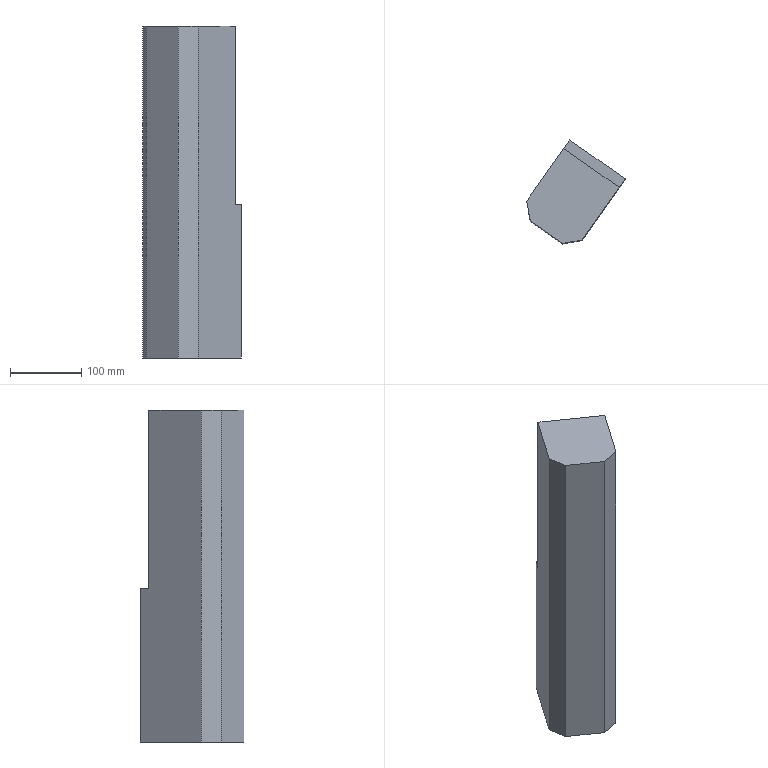Part | NX | features solid 2 | 1 solid | 22 faces | box 138.045 x 145.412 x 465 mm | volume 4926060 mm3 | plane 12 | cylinder 6 | cone 4 | commonest cylinder face diameters 16 x6
STEP:
#1=CARTESIAN_POINT('',(-184.572,-199.868,-589.062));
#2=VERTEX_POINT('',#1);
#3=CARTESIAN_POINT('',(-176.572,-199.868,-589.062));
#4=DIRECTION('',(0.,0.,-1.));
#5=DIRECTION('',(-1.,0.,0.));
#6=AXIS2_PLACEMENT_3D('',#3,#4,#5);
#7=CIRCLE('',#6,8.);
#8=EDGE_CURVE('',#2,#2,#7,.T.);
#9=ORIENTED_EDGE('',*,*,#8,.F.);
#10=EDGE_LOOP('',(#9));
#11=FACE_BOUND('',#10,.T.);
#12=CARTESIAN_POINT('',(-199.286,-147.842,-589.062));
#13=VERTEX_POINT('',#12);
#14=CARTESIAN_POINT('',(-207.286,-147.842,-589.062));
#15=DIRECTION('',(0.,0.,1.));
#16=DIRECTION('',(1.,0.,0.));
#17=AXIS2_PLACEMENT_3D('',#14,#15,#16);
#18=CIRCLE('',#17,8.);
#19=EDGE_CURVE('',#13,#13,#18,.T.);
#20=ORIENTED_EDGE('',*,*,#19,.T.);
#21=EDGE_LOOP('',(#20));
#22=FACE_BOUND('',#21,.T.);
#23=CARTESIAN_POINT('',(-236.569,-201.087,-589.062));
#24=VERTEX_POINT('',#23);
#25=CARTESIAN_POINT('',(-244.569,-201.087,-589.062));
#26=DIRECTION('',(0.,0.,1.));
#27=DIRECTION('',(1.,0.,0.));
#28=AXIS2_PLACEMENT_3D('',#25,#26,#27);
#29=CIRCLE('',#28,8.);
#30=EDGE_CURVE('',#24,#24,#29,.T.);
#31=ORIENTED_EDGE('',*,*,#30,.T.);
#32=EDGE_LOOP('',(#31));
#33=FACE_BOUND('',#32,.T.);
#34=CARTESIAN_POINT('',(-154.233,-179.389,-589.062));
#35=VERTEX_POINT('',#34);
#36=CARTESIAN_POINT('',(-162.233,-179.389,-589.062));
#37=DIRECTION('',(0.,0.,1.));
#38=DIRECTION('',(1.,0.,0.));
#39=AXIS2_PLACEMENT_3D('',#36,#37,#38);
#40=CIRCLE('',#39,8.);
#41=EDGE_CURVE('',#35,#35,#40,.T.);
#42=ORIENTED_EDGE('',*,*,#41,.T.);
#43=EDGE_LOOP('',(#42));
#44=FACE_BOUND('',#43,.T.);
#45=CARTESIAN_POINT('',(-191.515,-232.634,-589.062));
#46=VERTEX_POINT('',#45);
#47=CARTESIAN_POINT('',(-199.515,-232.634,-589.062));
#48=DIRECTION('',(0.,0.,1.));
#49=DIRECTION('',(1.,0.,0.));
#50=AXIS2_PLACEMENT_3D('',#47,#48,#49);
#51=CIRCLE('',#50,8.);
#52=EDGE_CURVE('',#46,#46,#51,.T.);
#53=ORIENTED_EDGE('',*,*,#52,.T.);
#54=EDGE_LOOP('',(#53));
#55=FACE_BOUND('',#54,.T.);
#56=CARTESIAN_POINT('',(-128.643,-166.286,-589.062));
#57=VERTEX_POINT('',#56);
#58=CARTESIAN_POINT('',(-188.868,-252.297,-589.062));
#59=VERTEX_POINT('',#58);
#60=CARTESIAN_POINT('',(-197.472,-264.584,-589.062));
#61=DIRECTION('',(-0.5736,-0.8192,0.));
#62=VECTOR('',#61,1000.);
#63=LINE('',#60,#62);
#64=EDGE_CURVE('',#57,#59,#63,.T.);
#65=ORIENTED_EDGE('',*,*,#64,.T.);
#66=CARTESIAN_POINT('',(-216.723,-257.209,-589.062));
#67=VERTEX_POINT('',#66);
#68=CARTESIAN_POINT('',(-188.868,-252.297,-589.062));
#69=DIRECTION('',(0.9848,0.1736,0.));
#70=VECTOR('',#69,1000.);
#71=LINE('',#68,#70);
#72=EDGE_CURVE('',#59,#67,#71,.F.);
#73=ORIENTED_EDGE('',*,*,#72,.T.);
#74=CARTESIAN_POINT('',(-261.776,-225.662,-589.062));
#75=VERTEX_POINT('',#74);
#76=CARTESIAN_POINT('',(-278.241,-214.133,-589.062));
#77=DIRECTION('',(0.8192,-0.5736,0.));
#78=VECTOR('',#77,1000.);
#79=LINE('',#76,#78);
#80=EDGE_CURVE('',#67,#75,#79,.F.);
#81=ORIENTED_EDGE('',*,*,#80,.T.);
#82=CARTESIAN_POINT('',(-266.688,-197.807,-589.062));
#83=VERTEX_POINT('',#82);
#84=CARTESIAN_POINT('',(-261.776,-225.662,-589.062));
#85=DIRECTION('',(0.1736,-0.9848,0.));
#86=VECTOR('',#85,1000.);
#87=LINE('',#84,#86);
#88=EDGE_CURVE('',#75,#83,#87,.F.);
#89=ORIENTED_EDGE('',*,*,#88,.T.);
#90=CARTESIAN_POINT('',(-206.462,-111.796,-589.062));
#91=VERTEX_POINT('',#90);
#92=CARTESIAN_POINT('',(-275.291,-210.095,-589.062));
#93=DIRECTION('',(0.5736,0.8192,0.));
#94=VECTOR('',#93,1000.);
#95=LINE('',#92,#94);
#96=EDGE_CURVE('',#91,#83,#95,.F.);
#97=ORIENTED_EDGE('',*,*,#96,.F.);
#98=CARTESIAN_POINT('',(-206.544,-111.739,-589.062));
#99=DIRECTION('',(0.8192,-0.5736,0.));
#100=VECTOR('',#99,1000.);
#101=LINE('',#98,#100);
#102=EDGE_CURVE('',#57,#91,#101,.F.);
#103=ORIENTED_EDGE('',*,*,#102,.F.);
#104=EDGE_LOOP('',(#65,#73,#81,#89,#97,#103));
#105=FACE_BOUND('',#104,.T.);
#106=CARTESIAN_POINT('',(-238.229,-180.609,-589.062));
#107=VERTEX_POINT('',#106);
#108=CARTESIAN_POINT('',(-230.229,-180.609,-589.062));
#109=DIRECTION('',(0.,0.,-1.));
#110=DIRECTION('',(-1.,0.,0.));
#111=AXIS2_PLACEMENT_3D('',#108,#109,#110);
#112=CIRCLE('',#111,8.);
#113=EDGE_CURVE('',#107,#107,#112,.T.);
#114=ORIENTED_EDGE('',*,*,#113,.F.);
#115=EDGE_LOOP('',(#114));
#116=FACE_BOUND('',#115,.T.);
#117=CARTESIAN_POINT('',(-275.373,-210.037,-589.062));
#118=DIRECTION('',(0.,0.,-1.));
#119=DIRECTION('',(0.5736,0.8192,0.));
#120=AXIS2_PLACEMENT_3D('',#117,#118,#119);
#121=PLANE('',#120);
#122=ADVANCED_FACE('',(#11,#22,#33,#44,#55,#105,#116),#121,.T.);
#123=CARTESIAN_POINT('',(-261.776,-225.662,-124.062));
#124=VERTEX_POINT('',#123);
#125=CARTESIAN_POINT('',(-216.723,-257.209,-124.062));
#126=VERTEX_POINT('',#125);
#127=CARTESIAN_POINT('',(-278.159,-214.19,-124.062));
#128=DIRECTION('',(0.8192,-0.5736,0.));
#129=VECTOR('',#128,1000.);
#130=LINE('',#127,#129);
#131=EDGE_CURVE('',#124,#126,#130,.T.);
#132=ORIENTED_EDGE('',*,*,#131,.T.);
#133=CARTESIAN_POINT('',(-188.868,-252.297,-124.062));
#134=VERTEX_POINT('',#133);
#135=CARTESIAN_POINT('',(-188.868,-252.297,-124.062));
#136=DIRECTION('',(0.9848,0.1736,0.));
#137=VECTOR('',#136,1000.);
#138=LINE('',#135,#137);
#139=EDGE_CURVE('',#126,#134,#138,.T.);
#140=ORIENTED_EDGE('',*,*,#139,.T.);
#141=CARTESIAN_POINT('',(-137.246,-178.573,-124.062));
#142=VERTEX_POINT('',#141);
#143=CARTESIAN_POINT('',(-48.342,-51.605,-124.062));
#144=DIRECTION('',(0.5736,0.8192,0.));
#145=VECTOR('',#144,1000.);
#146=LINE('',#143,#145);
#147=EDGE_CURVE('',#142,#134,#146,.F.);
#148=ORIENTED_EDGE('',*,*,#147,.F.);
#149=CARTESIAN_POINT('',(-215.066,-124.084,-124.062));
#150=VERTEX_POINT('',#149);
#151=CARTESIAN_POINT('',(-215.066,-124.084,-124.062));
#152=DIRECTION('',(0.8192,-0.5736,0.));
#153=VECTOR('',#152,1000.);
#154=LINE('',#151,#153);
#155=EDGE_CURVE('',#150,#142,#154,.T.);
#156=ORIENTED_EDGE('',*,*,#155,.F.);
#157=CARTESIAN_POINT('',(-266.688,-197.807,-124.062));
#158=VERTEX_POINT('',#157);
#159=CARTESIAN_POINT('',(-215.066,-124.084,-124.062));
#160=DIRECTION('',(-0.5736,-0.8192,0.));
#161=VECTOR('',#160,1000.);
#162=LINE('',#159,#161);
#163=EDGE_CURVE('',#150,#158,#162,.T.);
#164=ORIENTED_EDGE('',*,*,#163,.T.);
#165=CARTESIAN_POINT('',(-261.776,-225.662,-124.062));
#166=DIRECTION('',(0.1736,-0.9848,0.));
#167=VECTOR('',#166,1000.);
#168=LINE('',#165,#167);
#169=EDGE_CURVE('',#158,#124,#168,.T.);
#170=ORIENTED_EDGE('',*,*,#169,.T.);
#171=EDGE_LOOP('',(#132,#140,#148,#156,#164,#170));
#172=FACE_BOUND('',#171,.T.);
#173=CARTESIAN_POINT('',(-215.066,-124.084,-124.062));
#174=DIRECTION('',(0.,0.,-1.));
#175=DIRECTION('',(-0.5736,-0.8192,0.));
#176=AXIS2_PLACEMENT_3D('',#173,#174,#175);
#177=PLANE('',#176);
#178=ADVANCED_FACE('',(#172),#177,.F.);
#179=CARTESIAN_POINT('',(-137.246,-178.573,-374.062));
#180=VERTEX_POINT('',#179);
#181=CARTESIAN_POINT('',(-137.246,-178.573,-401.082));
#182=DIRECTION('',(0.,0.,1.));
#183=VECTOR('',#182,1000.);
#184=LINE('',#181,#183);
#185=EDGE_CURVE('',#142,#180,#184,.F.);
#186=ORIENTED_EDGE('',*,*,#185,.T.);
#187=CARTESIAN_POINT('',(-215.066,-124.084,-374.062));
#188=VERTEX_POINT('',#187);
#189=CARTESIAN_POINT('',(-215.066,-124.084,-374.062));
#190=DIRECTION('',(-0.8192,0.5736,0.));
#191=VECTOR('',#190,1000.);
#192=LINE('',#189,#191);
#193=EDGE_CURVE('',#180,#188,#192,.T.);
#194=ORIENTED_EDGE('',*,*,#193,.T.);
#195=CARTESIAN_POINT('',(-215.066,-124.084,-401.082));
#196=DIRECTION('',(0.,0.,-1.));
#197=VECTOR('',#196,1000.);
#198=LINE('',#195,#197);
#199=EDGE_CURVE('',#150,#188,#198,.T.);
#200=ORIENTED_EDGE('',*,*,#199,.F.);
#201=ORIENTED_EDGE('',*,*,#155,.T.);
#202=EDGE_LOOP('',(#186,#194,#200,#201));
#203=FACE_BOUND('',#202,.T.);
#204=CARTESIAN_POINT('',(-215.066,-124.084,-401.082));
#205=DIRECTION('',(-0.5736,-0.8192,0.));
#206=DIRECTION('',(0.8192,-0.5736,0.));
#207=AXIS2_PLACEMENT_3D('',#204,#205,#206);
#208=PLANE('',#207);
#209=ADVANCED_FACE('',(#203),#208,.F.);
#210=CARTESIAN_POINT('',(-128.643,-166.286,-374.062));
#211=VERTEX_POINT('',#210);
#212=CARTESIAN_POINT('',(-206.462,-111.796,-374.062));
#213=VERTEX_POINT('',#212);
#214=CARTESIAN_POINT('',(-153.217,-149.079,-374.062));
#215=DIRECTION('',(-0.8192,0.5736,0.));
#216=VECTOR('',#215,1000.);
#217=LINE('',#214,#216);
#218=EDGE_CURVE('',#211,#213,#217,.T.);
#219=ORIENTED_EDGE('',*,*,#218,.F.);
#220=CARTESIAN_POINT('',(-128.643,-166.286,-400.));
#221=DIRECTION('',(0.,0.,1.));
#222=VECTOR('',#221,1000.);
#223=LINE('',#220,#222);
#224=EDGE_CURVE('',#211,#57,#223,.F.);
#225=ORIENTED_EDGE('',*,*,#224,.T.);
#226=ORIENTED_EDGE('',*,*,#102,.T.);
#227=CARTESIAN_POINT('',(-206.462,-111.796,-401.082));
#228=DIRECTION('',(0.,0.,-1.));
#229=VECTOR('',#228,1000.);
#230=LINE('',#227,#229);
#231=EDGE_CURVE('',#213,#91,#230,.T.);
#232=ORIENTED_EDGE('',*,*,#231,.F.);
#233=EDGE_LOOP('',(#219,#225,#226,#232));
#234=FACE_BOUND('',#233,.T.);
#235=CARTESIAN_POINT('',(-153.217,-149.079,-461.082));
#236=DIRECTION('',(0.5736,0.8192,0.));
#237=DIRECTION('',(-0.8192,0.5736,0.));
#238=AXIS2_PLACEMENT_3D('',#235,#236,#237);
#239=PLANE('',#238);
#240=ADVANCED_FACE('',(#234),#239,.T.);
#241=ORIENTED_EDGE('',*,*,#96,.T.);
#242=CARTESIAN_POINT('',(-266.688,-197.807,-151.082));
#243=DIRECTION('',(0.,0.,1.));
#244=VECTOR('',#243,1000.);
#245=LINE('',#242,#244);
#246=EDGE_CURVE('',#83,#158,#245,.T.);
#247=ORIENTED_EDGE('',*,*,#246,.T.);
#248=ORIENTED_EDGE('',*,*,#163,.F.);
#249=ORIENTED_EDGE('',*,*,#199,.T.);
#250=CARTESIAN_POINT('',(-215.066,-124.084,-374.062));
#251=DIRECTION('',(-0.5736,-0.8192,0.));
#252=VECTOR('',#251,1000.);
#253=LINE('',#250,#252);
#254=EDGE_CURVE('',#213,#188,#253,.T.);
#255=ORIENTED_EDGE('',*,*,#254,.F.);
#256=ORIENTED_EDGE('',*,*,#231,.T.);
#257=EDGE_LOOP('',(#241,#247,#248,#249,#255,#256));
#258=FACE_BOUND('',#257,.T.);
#259=CARTESIAN_POINT('',(-215.066,-124.084,-151.082));
#260=DIRECTION('',(-0.8192,0.5736,0.));
#261=DIRECTION('',(-0.5736,-0.8192,0.));
#262=AXIS2_PLACEMENT_3D('',#259,#260,#261);
#263=PLANE('',#262);
#264=ADVANCED_FACE('',(#258),#263,.T.);
#265=ORIENTED_EDGE('',*,*,#80,.F.);
#266=CARTESIAN_POINT('',(-216.723,-257.209,-192.696));
#267=DIRECTION('',(0.,0.,1.));
#268=VECTOR('',#267,1000.);
#269=LINE('',#266,#268);
#270=EDGE_CURVE('',#67,#126,#269,.T.);
#271=ORIENTED_EDGE('',*,*,#270,.T.);
#272=ORIENTED_EDGE('',*,*,#131,.F.);
#273=CARTESIAN_POINT('',(-261.776,-225.662,-589.062));
#274=DIRECTION('',(0.,0.,-1.));
#275=VECTOR('',#274,1000.);
#276=LINE('',#273,#275);
#277=EDGE_CURVE('',#124,#75,#276,.T.);
#278=ORIENTED_EDGE('',*,*,#277,.T.);
#279=EDGE_LOOP('',(#265,#271,#272,#278));
#280=FACE_BOUND('',#279,.T.);
#281=CARTESIAN_POINT('',(-789.915,144.145,-192.696));
#282=DIRECTION('',(0.5736,0.8192,0.));
#283=DIRECTION('',(-0.8192,0.5736,0.));
#284=AXIS2_PLACEMENT_3D('',#281,#282,#283);
#285=PLANE('',#284);
#286=ADVANCED_FACE('',(#280),#285,.F.);
#287=CARTESIAN_POINT('',(-137.246,-178.573,-374.062));
#288=DIRECTION('',(0.5736,0.8192,0.));
#289=VECTOR('',#288,1000.);
#290=LINE('',#287,#289);
#291=EDGE_CURVE('',#211,#180,#290,.F.);
#292=ORIENTED_EDGE('',*,*,#291,.F.);
#293=ORIENTED_EDGE('',*,*,#218,.T.);
#294=ORIENTED_EDGE('',*,*,#254,.T.);
#295=ORIENTED_EDGE('',*,*,#193,.F.);
#296=EDGE_LOOP('',(#292,#293,#294,#295));
#297=FACE_BOUND('',#296,.T.);
#298=CARTESIAN_POINT('',(-161.821,-161.366,-374.062));
#299=DIRECTION('',(0.,0.,1.));
#300=DIRECTION('',(0.5736,0.8192,0.));
#301=AXIS2_PLACEMENT_3D('',#298,#299,#300);
#302=PLANE('',#301);
#303=ADVANCED_FACE('',(#297),#302,.T.);
#304=ORIENTED_EDGE('',*,*,#185,.F.);
#305=ORIENTED_EDGE('',*,*,#147,.T.);
#306=CARTESIAN_POINT('',(-188.868,-252.297,-400.));
#307=DIRECTION('',(0.,0.,1.));
#308=VECTOR('',#307,1000.);
#309=LINE('',#306,#308);
#310=EDGE_CURVE('',#134,#59,#309,.F.);
#311=ORIENTED_EDGE('',*,*,#310,.T.);
#312=ORIENTED_EDGE('',*,*,#64,.F.);
#313=ORIENTED_EDGE('',*,*,#224,.F.);
#314=ORIENTED_EDGE('',*,*,#291,.T.);
#315=EDGE_LOOP('',(#304,#305,#311,#312,#313,#314));
#316=FACE_BOUND('',#315,.T.);
#317=CARTESIAN_POINT('',(-48.342,-51.605,-400.));
#318=DIRECTION('',(0.8192,-0.5736,0.));
#319=DIRECTION('',(0.,0.,1.));
#320=AXIS2_PLACEMENT_3D('',#317,#318,#319);
#321=PLANE('',#320);
#322=ADVANCED_FACE('',(#316),#321,.T.);
#323=ORIENTED_EDGE('',*,*,#169,.F.);
#324=ORIENTED_EDGE('',*,*,#246,.F.);
#325=ORIENTED_EDGE('',*,*,#88,.F.);
#326=ORIENTED_EDGE('',*,*,#277,.F.);
#327=EDGE_LOOP('',(#323,#324,#325,#326));
#328=FACE_BOUND('',#327,.T.);
#329=CARTESIAN_POINT('',(-261.776,-225.662,-192.696));
#330=DIRECTION('',(-0.9848,-0.1736,0.));
#331=DIRECTION('',(0.1736,-0.9848,0.));
#332=AXIS2_PLACEMENT_3D('',#329,#330,#331);
#333=PLANE('',#332);
#334=ADVANCED_FACE('',(#328),#333,.T.);
#335=ORIENTED_EDGE('',*,*,#139,.F.);
#336=ORIENTED_EDGE('',*,*,#270,.F.);
#337=ORIENTED_EDGE('',*,*,#72,.F.);
#338=ORIENTED_EDGE('',*,*,#310,.F.);
#339=EDGE_LOOP('',(#335,#336,#337,#338));
#340=FACE_BOUND('',#339,.T.);
#341=CARTESIAN_POINT('',(-188.868,-252.297,-400.));
#342=DIRECTION('',(0.1736,-0.9848,0.));
#343=DIRECTION('',(0.9848,0.1736,0.));
#344=AXIS2_PLACEMENT_3D('',#341,#342,#343);
#345=PLANE('',#344);
#346=ADVANCED_FACE('',(#340),#345,.T.);
#347=CARTESIAN_POINT('',(-191.515,-232.634,-539.062));
#348=VERTEX_POINT('',#347);
#349=CARTESIAN_POINT('',(-199.515,-232.634,-539.062));
#350=DIRECTION('',(0.,0.,1.));
#351=DIRECTION('',(1.,0.,0.));
#352=AXIS2_PLACEMENT_3D('',#349,#350,#351);
#353=CIRCLE('',#352,8.);
#354=EDGE_CURVE('',#348,#348,#353,.T.);
#355=ORIENTED_EDGE('',*,*,#354,.F.);
#356=EDGE_LOOP('',(#355));
#357=FACE_BOUND('',#356,.T.);
#358=CARTESIAN_POINT('',(-199.515,-232.634,-534.256));
#359=VERTEX_POINT('',#358);
#360=VERTEX_LOOP('',#359);
#361=FACE_BOUND('',#360,.T.);
#362=CARTESIAN_POINT('',(-199.515,-232.634,-539.062));
#363=DIRECTION('',(0.,0.,-1.));
#364=DIRECTION('',(-1.,0.,0.));
#365=AXIS2_PLACEMENT_3D('',#362,#363,#364);
#366=CONICAL_SURFACE('',#365,8.,1.03);
#367=ADVANCED_FACE('',(#357,#361),#366,.F.);
#368=ORIENTED_EDGE('',*,*,#354,.T.);
#369=EDGE_LOOP('',(#368));
#370=FACE_BOUND('',#369,.T.);
#371=ORIENTED_EDGE('',*,*,#52,.F.);
#372=EDGE_LOOP('',(#371));
#373=FACE_BOUND('',#372,.T.);
#374=CARTESIAN_POINT('',(-199.515,-232.634,-589.062));
#375=DIRECTION('',(0.,0.,1.));
#376=DIRECTION('',(1.,0.,0.));
#377=AXIS2_PLACEMENT_3D('',#374,#375,#376);
#378=CYLINDRICAL_SURFACE('',#377,8.);
#379=ADVANCED_FACE('',(#370,#373),#378,.F.);
#380=CARTESIAN_POINT('',(-154.233,-179.389,-539.062));
#381=VERTEX_POINT('',#380);
#382=CARTESIAN_POINT('',(-162.233,-179.389,-539.062));
#383=DIRECTION('',(0.,0.,1.));
#384=DIRECTION('',(1.,0.,0.));
#385=AXIS2_PLACEMENT_3D('',#382,#383,#384);
#386=CIRCLE('',#385,8.);
#387=EDGE_CURVE('',#381,#381,#386,.T.);
#388=ORIENTED_EDGE('',*,*,#387,.F.);
#389=EDGE_LOOP('',(#388));
#390=FACE_BOUND('',#389,.T.);
#391=CARTESIAN_POINT('',(-162.233,-179.389,-534.256));
#392=VERTEX_POINT('',#391);
#393=VERTEX_LOOP('',#392);
#394=FACE_BOUND('',#393,.T.);
#395=CARTESIAN_POINT('',(-162.233,-179.389,-539.062));
#396=DIRECTION('',(0.,0.,-1.));
#397=DIRECTION('',(-1.,0.,0.));
#398=AXIS2_PLACEMENT_3D('',#395,#396,#397);
#399=CONICAL_SURFACE('',#398,8.,1.03);
#400=ADVANCED_FACE('',(#390,#394),#399,.F.);
#401=ORIENTED_EDGE('',*,*,#387,.T.);
#402=EDGE_LOOP('',(#401));
#403=FACE_BOUND('',#402,.T.);
#404=ORIENTED_EDGE('',*,*,#41,.F.);
#405=EDGE_LOOP('',(#404));
#406=FACE_BOUND('',#405,.T.);
#407=CARTESIAN_POINT('',(-162.233,-179.389,-589.062));
#408=DIRECTION('',(0.,0.,1.));
#409=DIRECTION('',(1.,0.,0.));
#410=AXIS2_PLACEMENT_3D('',#407,#408,#409);
#411=CYLINDRICAL_SURFACE('',#410,8.);
#412=ADVANCED_FACE('',(#403,#406),#411,.F.);
#413=CARTESIAN_POINT('',(-236.569,-201.087,-539.062));
#414=VERTEX_POINT('',#413);
#415=CARTESIAN_POINT('',(-244.569,-201.087,-539.062));
#416=DIRECTION('',(0.,0.,1.));
#417=DIRECTION('',(1.,0.,0.));
#418=AXIS2_PLACEMENT_3D('',#415,#416,#417);
#419=CIRCLE('',#418,8.);
#420=EDGE_CURVE('',#414,#414,#419,.T.);
#421=ORIENTED_EDGE('',*,*,#420,.F.);
#422=EDGE_LOOP('',(#421));
#423=FACE_BOUND('',#422,.T.);
#424=CARTESIAN_POINT('',(-244.569,-201.087,-534.256));
#425=VERTEX_POINT('',#424);
#426=VERTEX_LOOP('',#425);
#427=FACE_BOUND('',#426,.T.);
#428=CARTESIAN_POINT('',(-244.569,-201.087,-539.062));
#429=DIRECTION('',(0.,0.,-1.));
#430=DIRECTION('',(-1.,0.,0.));
#431=AXIS2_PLACEMENT_3D('',#428,#429,#430);
#432=CONICAL_SURFACE('',#431,8.,1.03);
#433=ADVANCED_FACE('',(#423,#427),#432,.F.);
#434=ORIENTED_EDGE('',*,*,#420,.T.);
#435=EDGE_LOOP('',(#434));
#436=FACE_BOUND('',#435,.T.);
#437=ORIENTED_EDGE('',*,*,#30,.F.);
#438=EDGE_LOOP('',(#437));
#439=FACE_BOUND('',#438,.T.);
#440=CARTESIAN_POINT('',(-244.569,-201.087,-589.062));
#441=DIRECTION('',(0.,0.,1.));
#442=DIRECTION('',(1.,0.,0.));
#443=AXIS2_PLACEMENT_3D('',#440,#441,#442);
#444=CYLINDRICAL_SURFACE('',#443,8.);
#445=ADVANCED_FACE('',(#436,#439),#444,.F.);
#446=CARTESIAN_POINT('',(-199.286,-147.842,-539.062));
#447=VERTEX_POINT('',#446);
#448=CARTESIAN_POINT('',(-207.286,-147.842,-539.062));
#449=DIRECTION('',(0.,0.,1.));
#450=DIRECTION('',(1.,0.,0.));
#451=AXIS2_PLACEMENT_3D('',#448,#449,#450);
#452=CIRCLE('',#451,8.);
#453=EDGE_CURVE('',#447,#447,#452,.T.);
#454=ORIENTED_EDGE('',*,*,#453,.F.);
#455=EDGE_LOOP('',(#454));
#456=FACE_BOUND('',#455,.T.);
#457=CARTESIAN_POINT('',(-207.286,-147.842,-534.256));
#458=VERTEX_POINT('',#457);
#459=VERTEX_LOOP('',#458);
#460=FACE_BOUND('',#459,.T.);
#461=CARTESIAN_POINT('',(-207.286,-147.842,-539.062));
#462=DIRECTION('',(0.,0.,-1.));
#463=DIRECTION('',(-1.,0.,0.));
#464=AXIS2_PLACEMENT_3D('',#461,#462,#463);
#465=CONICAL_SURFACE('',#464,8.,1.03);
#466=ADVANCED_FACE('',(#456,#460),#465,.F.);
#467=ORIENTED_EDGE('',*,*,#453,.T.);
#468=EDGE_LOOP('',(#467));
#469=FACE_BOUND('',#468,.T.);
#470=ORIENTED_EDGE('',*,*,#19,.F.);
#471=EDGE_LOOP('',(#470));
#472=FACE_BOUND('',#471,.T.);
#473=CARTESIAN_POINT('',(-207.286,-147.842,-589.062));
#474=DIRECTION('',(0.,0.,1.));
#475=DIRECTION('',(1.,0.,0.));
#476=AXIS2_PLACEMENT_3D('',#473,#474,#475);
#477=CYLINDRICAL_SURFACE('',#476,8.);
#478=ADVANCED_FACE('',(#469,#472),#477,.F.);
#479=CARTESIAN_POINT('',(-184.572,-199.868,-559.062));
#480=VERTEX_POINT('',#479);
#481=CARTESIAN_POINT('',(-176.572,-199.868,-559.062));
#482=DIRECTION('',(0.,0.,-1.));
#483=DIRECTION('',(-1.,0.,0.));
#484=AXIS2_PLACEMENT_3D('',#481,#482,#483);
#485=CIRCLE('',#484,8.);
#486=EDGE_CURVE('',#480,#480,#485,.T.);
#487=ORIENTED_EDGE('',*,*,#486,.F.);
#488=EDGE_LOOP('',(#487));
#489=FACE_BOUND('',#488,.T.);
#490=ORIENTED_EDGE('',*,*,#8,.T.);
#491=EDGE_LOOP('',(#490));
#492=FACE_BOUND('',#491,.T.);
#493=CARTESIAN_POINT('',(-176.572,-199.868,-639.062));
#494=DIRECTION('',(0.,0.,1.));
#495=DIRECTION('',(1.,0.,0.));
#496=AXIS2_PLACEMENT_3D('',#493,#494,#495);
#497=CYLINDRICAL_SURFACE('',#496,8.);
#498=ADVANCED_FACE('',(#489,#492),#497,.F.);
#499=ORIENTED_EDGE('',*,*,#486,.T.);
#500=EDGE_LOOP('',(#499));
#501=FACE_BOUND('',#500,.T.);
#502=CARTESIAN_POINT('',(-176.572,-199.868,-559.062));
#503=DIRECTION('',(0.,0.,-1.));
#504=DIRECTION('',(-1.,0.,0.));
#505=AXIS2_PLACEMENT_3D('',#502,#503,#504);
#506=PLANE('',#505);
#507=ADVANCED_FACE('',(#501),#506,.T.);
#508=CARTESIAN_POINT('',(-238.229,-180.609,-559.062));
#509=VERTEX_POINT('',#508);
#510=CARTESIAN_POINT('',(-230.229,-180.609,-559.062));
#511=DIRECTION('',(0.,0.,-1.));
#512=DIRECTION('',(-1.,0.,0.));
#513=AXIS2_PLACEMENT_3D('',#510,#511,#512);
#514=CIRCLE('',#513,8.);
#515=EDGE_CURVE('',#509,#509,#514,.T.);
#516=ORIENTED_EDGE('',*,*,#515,.F.);
#517=EDGE_LOOP('',(#516));
#518=FACE_BOUND('',#517,.T.);
#519=ORIENTED_EDGE('',*,*,#113,.T.);
#520=EDGE_LOOP('',(#519));
#521=FACE_BOUND('',#520,.T.);
#522=CARTESIAN_POINT('',(-230.229,-180.609,-639.062));
#523=DIRECTION('',(0.,0.,1.));
#524=DIRECTION('',(1.,0.,0.));
#525=AXIS2_PLACEMENT_3D('',#522,#523,#524);
#526=CYLINDRICAL_SURFACE('',#525,8.);
#527=ADVANCED_FACE('',(#518,#521),#526,.F.);
#528=ORIENTED_EDGE('',*,*,#515,.T.);
#529=EDGE_LOOP('',(#528));
#530=FACE_BOUND('',#529,.T.);
#531=CARTESIAN_POINT('',(-230.229,-180.609,-559.062));
#532=DIRECTION('',(0.,0.,-1.));
#533=DIRECTION('',(-1.,0.,0.));
#534=AXIS2_PLACEMENT_3D('',#531,#532,#533);
#535=PLANE('',#534);
#536=ADVANCED_FACE('',(#530),#535,.T.);
#537=CLOSED_SHELL('',(#122,#178,#209,#240,#264,#286,#303,#322,#334,#346,#367,#379,#400,#412,#433,#445,#466,#478,#498,#507,#527,#536));
#538=MANIFOLD_SOLID_BREP('',#537);
#539=(LENGTH_UNIT()NAMED_UNIT(*)SI_UNIT(.MILLI.,.METRE.));
#540=UNCERTAINTY_MEASURE_WITH_UNIT(LENGTH_MEASURE(0.00001),#539,'','');
#541=(NAMED_UNIT(*)PLANE_ANGLE_UNIT()SI_UNIT($,.RADIAN.));
#542=(NAMED_UNIT(*)SI_UNIT($,.STERADIAN.)SOLID_ANGLE_UNIT());
#543=(GEOMETRIC_REPRESENTATION_CONTEXT(3)GLOBAL_UNCERTAINTY_ASSIGNED_CONTEXT((#540))GLOBAL_UNIT_ASSIGNED_CONTEXT((#539,#541,#542))REPRESENTATION_CONTEXT('',''));
#544=ADVANCED_BREP_SHAPE_REPRESENTATION('',(#538),#543);